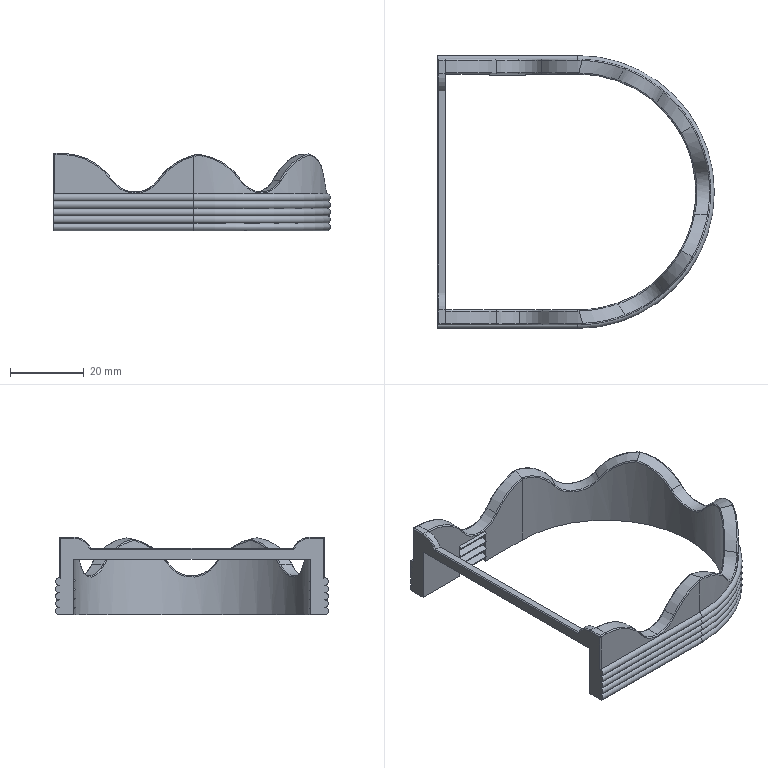Part | SolidWorks | features ICE 8, Chamfer 3, ExtruRefSurface 2, Fillet 2, MirrorPattern 2, SurfCut 2, CurvePattern 1, LPattern 1, Stock 1 | 1 solid | 154 faces | box 75 x 74 x 21 mm | volume 13589 mm3 | plane 69 | cylinder 40 | spline 22 | torus 21 | sphere 2 | commonest cylinder face diameters 2 x12 33.595 x10 0.6 x8 15 x6 10 x2 64 x1